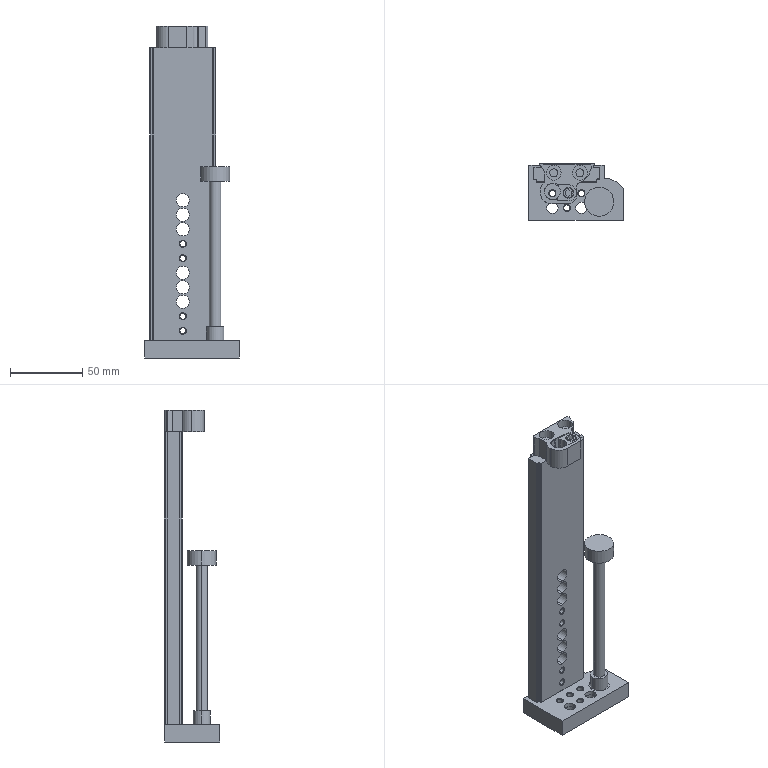Part | SolidWorks | features RevCut 22, RefAxis 18, ICE 12, 3DProfileFeature 6, Revolution 2, Extrusion 1 | 1 solid | 262 faces | box 65 x 38.5 x 229 mm | volume 144902 mm3 | plane 106 | cylinder 103 | cone 47 | torus 6 | commonest cylinder face diameters 7 x19 4.134 x18 9 x12 0.4 x6 8 x6 10 x6